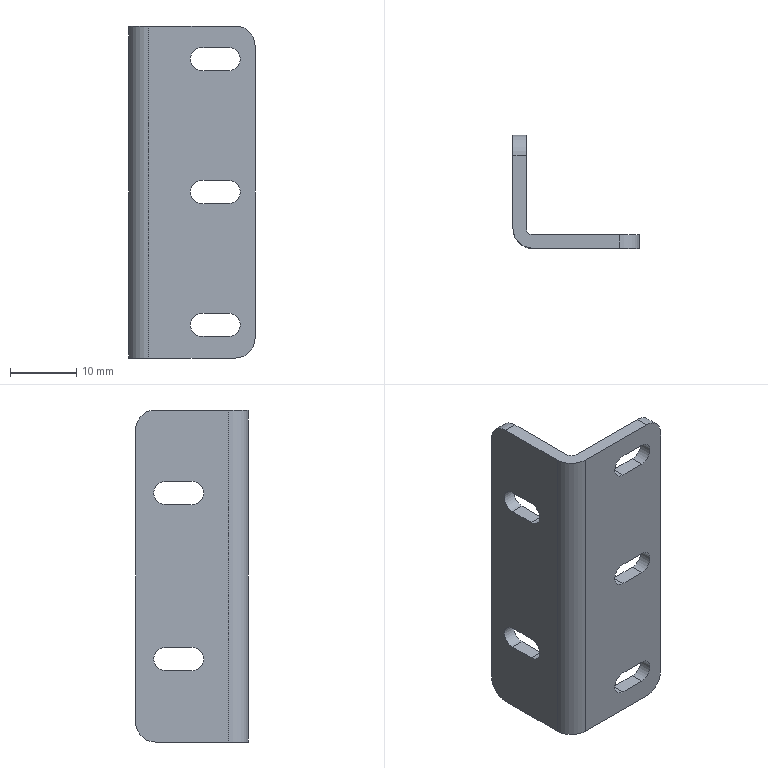Part | SolidWorks | features Fillet 3, ICE 2, ExtruThin 1 | 1 solid | 34 faces | box 19 x 17 x 50 mm | volume 3062 mm3 | plane 18 | cylinder 16 | commonest cylinder face diameters 3.5 x10 6 x5 2 x1
STEP:
#1=CARTESIAN_POINT('',(13.,-2.,18.25));
#2=VERTEX_POINT('',#1);
#3=CARTESIAN_POINT('',(9.,-2.,18.25));
#4=VERTEX_POINT('',#3);
#5=CARTESIAN_POINT('',(0.,-2.,18.25));
#6=DIRECTION('',(-1.,0.,0.));
#7=VECTOR('',#6,1000.);
#8=LINE('',#5,#7);
#9=EDGE_CURVE('',#2,#4,#8,.T.);
#10=ORIENTED_EDGE('',*,*,#9,.T.);
#11=CARTESIAN_POINT('',(9.,-2.,21.75));
#12=VERTEX_POINT('',#11);
#13=CARTESIAN_POINT('',(9.,-2.,20.));
#14=DIRECTION('',(0.,1.,0.));
#15=DIRECTION('',(0.,0.,1.));
#16=AXIS2_PLACEMENT_3D('',#13,#14,#15);
#17=CIRCLE('',#16,1.75);
#18=EDGE_CURVE('',#4,#12,#17,.T.);
#19=ORIENTED_EDGE('',*,*,#18,.T.);
#20=CARTESIAN_POINT('',(13.,-2.,21.75));
#21=VERTEX_POINT('',#20);
#22=CARTESIAN_POINT('',(0.,-2.,21.75));
#23=DIRECTION('',(1.,0.,0.));
#24=VECTOR('',#23,1000.);
#25=LINE('',#22,#24);
#26=EDGE_CURVE('',#12,#21,#25,.T.);
#27=ORIENTED_EDGE('',*,*,#26,.T.);
#28=CARTESIAN_POINT('',(13.,-2.,20.));
#29=DIRECTION('',(0.,1.,0.));
#30=DIRECTION('',(0.,0.,1.));
#31=AXIS2_PLACEMENT_3D('',#28,#29,#30);
#32=CIRCLE('',#31,1.75);
#33=EDGE_CURVE('',#21,#2,#32,.T.);
#34=ORIENTED_EDGE('',*,*,#33,.T.);
#35=EDGE_LOOP('',(#10,#19,#27,#34));
#36=FACE_BOUND('',#35,.T.);
#37=CARTESIAN_POINT('',(13.,-2.,-1.75));
#38=VERTEX_POINT('',#37);
#39=CARTESIAN_POINT('',(9.,-2.,-1.75));
#40=VERTEX_POINT('',#39);
#41=CARTESIAN_POINT('',(0.,-2.,-1.75));
#42=DIRECTION('',(-1.,0.,0.));
#43=VECTOR('',#42,1000.);
#44=LINE('',#41,#43);
#45=EDGE_CURVE('',#38,#40,#44,.T.);
#46=ORIENTED_EDGE('',*,*,#45,.T.);
#47=CARTESIAN_POINT('',(9.,-2.,1.75));
#48=VERTEX_POINT('',#47);
#49=CARTESIAN_POINT('',(9.,-2.,0.));
#50=DIRECTION('',(0.,1.,0.));
#51=DIRECTION('',(0.,0.,1.));
#52=AXIS2_PLACEMENT_3D('',#49,#50,#51);
#53=CIRCLE('',#52,1.75);
#54=EDGE_CURVE('',#40,#48,#53,.T.);
#55=ORIENTED_EDGE('',*,*,#54,.T.);
#56=CARTESIAN_POINT('',(13.,-2.,1.75));
#57=VERTEX_POINT('',#56);
#58=CARTESIAN_POINT('',(0.,-2.,1.75));
#59=DIRECTION('',(1.,0.,0.));
#60=VECTOR('',#59,1000.);
#61=LINE('',#58,#60);
#62=EDGE_CURVE('',#48,#57,#61,.T.);
#63=ORIENTED_EDGE('',*,*,#62,.T.);
#64=CARTESIAN_POINT('',(13.,-2.,0.));
#65=DIRECTION('',(0.,1.,0.));
#66=DIRECTION('',(0.,0.,1.));
#67=AXIS2_PLACEMENT_3D('',#64,#65,#66);
#68=CIRCLE('',#67,1.75);
#69=EDGE_CURVE('',#57,#38,#68,.T.);
#70=ORIENTED_EDGE('',*,*,#69,.T.);
#71=EDGE_LOOP('',(#46,#55,#63,#70));
#72=FACE_BOUND('',#71,.T.);
#73=CARTESIAN_POINT('',(13.,-2.,-21.75));
#74=VERTEX_POINT('',#73);
#75=CARTESIAN_POINT('',(9.,-2.,-21.75));
#76=VERTEX_POINT('',#75);
#77=CARTESIAN_POINT('',(0.,-2.,-21.75));
#78=DIRECTION('',(-1.,0.,0.));
#79=VECTOR('',#78,1000.);
#80=LINE('',#77,#79);
#81=EDGE_CURVE('',#74,#76,#80,.T.);
#82=ORIENTED_EDGE('',*,*,#81,.T.);
#83=CARTESIAN_POINT('',(9.,-2.,-18.25));
#84=VERTEX_POINT('',#83);
#85=CARTESIAN_POINT('',(9.,-2.,-20.));
#86=DIRECTION('',(0.,1.,0.));
#87=DIRECTION('',(0.,0.,1.));
#88=AXIS2_PLACEMENT_3D('',#85,#86,#87);
#89=CIRCLE('',#88,1.75);
#90=EDGE_CURVE('',#76,#84,#89,.T.);
#91=ORIENTED_EDGE('',*,*,#90,.T.);
#92=CARTESIAN_POINT('',(13.,-2.,-18.25));
#93=VERTEX_POINT('',#92);
#94=CARTESIAN_POINT('',(0.,-2.,-18.25));
#95=DIRECTION('',(1.,0.,0.));
#96=VECTOR('',#95,1000.);
#97=LINE('',#94,#96);
#98=EDGE_CURVE('',#84,#93,#97,.T.);
#99=ORIENTED_EDGE('',*,*,#98,.T.);
#100=CARTESIAN_POINT('',(13.,-2.,-20.));
#101=DIRECTION('',(0.,1.,0.));
#102=DIRECTION('',(0.,0.,1.));
#103=AXIS2_PLACEMENT_3D('',#100,#101,#102);
#104=CIRCLE('',#103,1.75);
#105=EDGE_CURVE('',#93,#74,#104,.T.);
#106=ORIENTED_EDGE('',*,*,#105,.T.);
#107=EDGE_LOOP('',(#82,#91,#99,#106));
#108=FACE_BOUND('',#107,.T.);
#109=CARTESIAN_POINT('',(1.,-2.,25.));
#110=VERTEX_POINT('',#109);
#111=CARTESIAN_POINT('',(14.,-2.,25.));
#112=VERTEX_POINT('',#111);
#113=CARTESIAN_POINT('',(0.,-2.,25.));
#114=DIRECTION('',(1.,0.,0.));
#115=VECTOR('',#114,1000.);
#116=LINE('',#113,#115);
#117=EDGE_CURVE('',#110,#112,#116,.T.);
#118=ORIENTED_EDGE('',*,*,#117,.F.);
#119=CARTESIAN_POINT('',(1.,-2.,-25.));
#120=VERTEX_POINT('',#119);
#121=CARTESIAN_POINT('',(1.,-2.,25.));
#122=DIRECTION('',(0.,0.,-1.));
#123=VECTOR('',#122,1000.);
#124=LINE('',#121,#123);
#125=EDGE_CURVE('',#110,#120,#124,.T.);
#126=ORIENTED_EDGE('',*,*,#125,.T.);
#127=CARTESIAN_POINT('',(14.,-2.,-25.));
#128=VERTEX_POINT('',#127);
#129=CARTESIAN_POINT('',(0.,-2.,-25.));
#130=DIRECTION('',(1.,0.,0.));
#131=VECTOR('',#130,1000.);
#132=LINE('',#129,#131);
#133=EDGE_CURVE('',#120,#128,#132,.T.);
#134=ORIENTED_EDGE('',*,*,#133,.T.);
#135=CARTESIAN_POINT('',(17.,-2.,-22.));
#136=VERTEX_POINT('',#135);
#137=CARTESIAN_POINT('',(14.,-2.,-22.));
#138=DIRECTION('',(0.,-1.,0.));
#139=DIRECTION('',(0.,0.,1.));
#140=AXIS2_PLACEMENT_3D('',#137,#138,#139);
#141=CIRCLE('',#140,3.);
#142=EDGE_CURVE('',#128,#136,#141,.T.);
#143=ORIENTED_EDGE('',*,*,#142,.T.);
#144=CARTESIAN_POINT('',(17.,-2.,22.));
#145=VERTEX_POINT('',#144);
#146=CARTESIAN_POINT('',(17.,-2.,25.));
#147=DIRECTION('',(0.,0.,-1.));
#148=VECTOR('',#147,1000.);
#149=LINE('',#146,#148);
#150=EDGE_CURVE('',#145,#136,#149,.T.);
#151=ORIENTED_EDGE('',*,*,#150,.F.);
#152=CARTESIAN_POINT('',(14.,-2.,22.));
#153=DIRECTION('',(0.,-1.,0.));
#154=DIRECTION('',(0.,0.,1.));
#155=AXIS2_PLACEMENT_3D('',#152,#153,#154);
#156=CIRCLE('',#155,3.);
#157=EDGE_CURVE('',#145,#112,#156,.T.);
#158=ORIENTED_EDGE('',*,*,#157,.T.);
#159=EDGE_LOOP('',(#118,#126,#134,#143,#151,#158));
#160=FACE_OUTER_BOUND('',#159,.T.);
#161=CARTESIAN_POINT('',(0.,-2.,25.));
#162=DIRECTION('',(0.,1.,0.));
#163=DIRECTION('',(0.,0.,1.));
#164=AXIS2_PLACEMENT_3D('',#161,#162,#163);
#165=PLANE('',#164);
#166=ADVANCED_FACE('',(#36,#72,#108,#160),#165,.F.);
#167=CARTESIAN_POINT('',(17.,0.,22.));
#168=VERTEX_POINT('',#167);
#169=CARTESIAN_POINT('',(17.,0.,-22.));
#170=VERTEX_POINT('',#169);
#171=CARTESIAN_POINT('',(17.,0.,25.));
#172=DIRECTION('',(0.,0.,-1.));
#173=VECTOR('',#172,1000.);
#174=LINE('',#171,#173);
#175=EDGE_CURVE('',#168,#170,#174,.T.);
#176=ORIENTED_EDGE('',*,*,#175,.F.);
#177=CARTESIAN_POINT('',(17.,-2.,22.));
#178=DIRECTION('',(0.,-1.,0.));
#179=VECTOR('',#178,1000.);
#180=LINE('',#177,#179);
#181=EDGE_CURVE('',#168,#145,#180,.T.);
#182=ORIENTED_EDGE('',*,*,#181,.T.);
#183=ORIENTED_EDGE('',*,*,#150,.T.);
#184=CARTESIAN_POINT('',(17.,0.,-22.));
#185=DIRECTION('',(0.,1.,0.));
#186=VECTOR('',#185,1000.);
#187=LINE('',#184,#186);
#188=EDGE_CURVE('',#136,#170,#187,.T.);
#189=ORIENTED_EDGE('',*,*,#188,.T.);
#190=EDGE_LOOP('',(#176,#182,#183,#189));
#191=FACE_OUTER_BOUND('',#190,.T.);
#192=CARTESIAN_POINT('',(17.,0.,25.));
#193=DIRECTION('',(1.,0.,0.));
#194=DIRECTION('',(0.,0.,-1.));
#195=AXIS2_PLACEMENT_3D('',#192,#193,#194);
#196=PLANE('',#195);
#197=ADVANCED_FACE('',(#191),#196,.T.);
#198=CARTESIAN_POINT('',(9.,0.,18.25));
#199=VERTEX_POINT('',#198);
#200=CARTESIAN_POINT('',(9.,0.,21.75));
#201=VERTEX_POINT('',#200);
#202=CARTESIAN_POINT('',(9.,0.,20.));
#203=DIRECTION('',(0.,1.,0.));
#204=DIRECTION('',(0.,0.,-1.));
#205=AXIS2_PLACEMENT_3D('',#202,#203,#204);
#206=CIRCLE('',#205,1.75);
#207=EDGE_CURVE('',#199,#201,#206,.T.);
#208=ORIENTED_EDGE('',*,*,#207,.F.);
#209=CARTESIAN_POINT('',(13.,0.,18.25));
#210=VERTEX_POINT('',#209);
#211=CARTESIAN_POINT('',(9.,0.,18.25));
#212=DIRECTION('',(-1.,0.,0.));
#213=VECTOR('',#212,1000.);
#214=LINE('',#211,#213);
#215=EDGE_CURVE('',#210,#199,#214,.T.);
#216=ORIENTED_EDGE('',*,*,#215,.F.);
#217=CARTESIAN_POINT('',(13.,0.,21.75));
#218=VERTEX_POINT('',#217);
#219=CARTESIAN_POINT('',(13.,0.,20.));
#220=DIRECTION('',(0.,1.,0.));
#221=DIRECTION('',(0.,0.,-1.));
#222=AXIS2_PLACEMENT_3D('',#219,#220,#221);
#223=CIRCLE('',#222,1.75);
#224=EDGE_CURVE('',#218,#210,#223,.T.);
#225=ORIENTED_EDGE('',*,*,#224,.F.);
#226=CARTESIAN_POINT('',(9.,0.,21.75));
#227=DIRECTION('',(1.,0.,0.));
#228=VECTOR('',#227,1000.);
#229=LINE('',#226,#228);
#230=EDGE_CURVE('',#201,#218,#229,.T.);
#231=ORIENTED_EDGE('',*,*,#230,.F.);
#232=EDGE_LOOP('',(#208,#216,#225,#231));
#233=FACE_BOUND('',#232,.T.);
#234=CARTESIAN_POINT('',(9.,0.,-1.75));
#235=VERTEX_POINT('',#234);
#236=CARTESIAN_POINT('',(9.,0.,1.75));
#237=VERTEX_POINT('',#236);
#238=CARTESIAN_POINT('',(9.,0.,0.));
#239=DIRECTION('',(0.,1.,0.));
#240=DIRECTION('',(0.,0.,1.));
#241=AXIS2_PLACEMENT_3D('',#238,#239,#240);
#242=CIRCLE('',#241,1.75);
#243=EDGE_CURVE('',#235,#237,#242,.T.);
#244=ORIENTED_EDGE('',*,*,#243,.F.);
#245=CARTESIAN_POINT('',(13.,0.,-1.75));
#246=VERTEX_POINT('',#245);
#247=CARTESIAN_POINT('',(9.,0.,-1.75));
#248=DIRECTION('',(-1.,0.,0.));
#249=VECTOR('',#248,1000.);
#250=LINE('',#247,#249);
#251=EDGE_CURVE('',#246,#235,#250,.T.);
#252=ORIENTED_EDGE('',*,*,#251,.F.);
#253=CARTESIAN_POINT('',(13.,0.,1.75));
#254=VERTEX_POINT('',#253);
#255=CARTESIAN_POINT('',(13.,0.,0.));
#256=DIRECTION('',(0.,1.,0.));
#257=DIRECTION('',(0.,0.,1.));
#258=AXIS2_PLACEMENT_3D('',#255,#256,#257);
#259=CIRCLE('',#258,1.75);
#260=EDGE_CURVE('',#254,#246,#259,.T.);
#261=ORIENTED_EDGE('',*,*,#260,.F.);
#262=CARTESIAN_POINT('',(9.,0.,1.75));
#263=DIRECTION('',(1.,0.,0.));
#264=VECTOR('',#263,1000.);
#265=LINE('',#262,#264);
#266=EDGE_CURVE('',#237,#254,#265,.T.);
#267=ORIENTED_EDGE('',*,*,#266,.F.);
#268=EDGE_LOOP('',(#244,#252,#261,#267));
#269=FACE_BOUND('',#268,.T.);
#270=CARTESIAN_POINT('',(9.,0.,-21.75));
#271=VERTEX_POINT('',#270);
#272=CARTESIAN_POINT('',(9.,0.,-18.25));
#273=VERTEX_POINT('',#272);
#274=CARTESIAN_POINT('',(9.,0.,-20.));
#275=DIRECTION('',(0.,1.,0.));
#276=DIRECTION('',(0.,0.,1.));
#277=AXIS2_PLACEMENT_3D('',#274,#275,#276);
#278=CIRCLE('',#277,1.75);
#279=EDGE_CURVE('',#271,#273,#278,.T.);
#280=ORIENTED_EDGE('',*,*,#279,.F.);
#281=CARTESIAN_POINT('',(13.,0.,-21.75));
#282=VERTEX_POINT('',#281);
#283=CARTESIAN_POINT('',(9.,0.,-21.75));
#284=DIRECTION('',(-1.,0.,0.));
#285=VECTOR('',#284,1000.);
#286=LINE('',#283,#285);
#287=EDGE_CURVE('',#282,#271,#286,.T.);
#288=ORIENTED_EDGE('',*,*,#287,.F.);
#289=CARTESIAN_POINT('',(13.,0.,-18.25));
#290=VERTEX_POINT('',#289);
#291=CARTESIAN_POINT('',(13.,0.,-20.));
#292=DIRECTION('',(0.,1.,0.));
#293=DIRECTION('',(0.,0.,1.));
#294=AXIS2_PLACEMENT_3D('',#291,#292,#293);
#295=CIRCLE('',#294,1.75);
#296=EDGE_CURVE('',#290,#282,#295,.T.);
#297=ORIENTED_EDGE('',*,*,#296,.F.);
#298=CARTESIAN_POINT('',(9.,0.,-18.25));
#299=DIRECTION('',(1.,0.,0.));
#300=VECTOR('',#299,1000.);
#301=LINE('',#298,#300);
#302=EDGE_CURVE('',#273,#290,#301,.T.);
#303=ORIENTED_EDGE('',*,*,#302,.F.);
#304=EDGE_LOOP('',(#280,#288,#297,#303));
#305=FACE_BOUND('',#304,.T.);
#306=CARTESIAN_POINT('',(1.,0.,-25.));
#307=VERTEX_POINT('',#306);
#308=CARTESIAN_POINT('',(14.,0.,-25.));
#309=VERTEX_POINT('',#308);
#310=CARTESIAN_POINT('',(0.,0.,-25.));
#311=DIRECTION('',(1.,0.,0.));
#312=VECTOR('',#311,1000.);
#313=LINE('',#310,#312);
#314=EDGE_CURVE('',#307,#309,#313,.T.);
#315=ORIENTED_EDGE('',*,*,#314,.F.);
#316=CARTESIAN_POINT('',(1.,0.,25.));
#317=VERTEX_POINT('',#316);
#318=CARTESIAN_POINT('',(1.,0.,25.));
#319=DIRECTION('',(0.,0.,1.));
#320=VECTOR('',#319,1000.);
#321=LINE('',#318,#320);
#322=EDGE_CURVE('',#307,#317,#321,.T.);
#323=ORIENTED_EDGE('',*,*,#322,.T.);
#324=CARTESIAN_POINT('',(14.,0.,25.));
#325=VERTEX_POINT('',#324);
#326=CARTESIAN_POINT('',(0.,0.,25.));
#327=DIRECTION('',(1.,0.,0.));
#328=VECTOR('',#327,1000.);
#329=LINE('',#326,#328);
#330=EDGE_CURVE('',#317,#325,#329,.T.);
#331=ORIENTED_EDGE('',*,*,#330,.T.);
#332=CARTESIAN_POINT('',(14.,0.,22.));
#333=DIRECTION('',(0.,1.,0.));
#334=DIRECTION('',(0.,0.,1.));
#335=AXIS2_PLACEMENT_3D('',#332,#333,#334);
#336=CIRCLE('',#335,3.);
#337=EDGE_CURVE('',#325,#168,#336,.T.);
#338=ORIENTED_EDGE('',*,*,#337,.T.);
#339=ORIENTED_EDGE('',*,*,#175,.T.);
#340=CARTESIAN_POINT('',(14.,0.,-22.));
#341=DIRECTION('',(0.,1.,0.));
#342=DIRECTION('',(0.,0.,1.));
#343=AXIS2_PLACEMENT_3D('',#340,#341,#342);
#344=CIRCLE('',#343,3.);
#345=EDGE_CURVE('',#170,#309,#344,.T.);
#346=ORIENTED_EDGE('',*,*,#345,.T.);
#347=EDGE_LOOP('',(#315,#323,#331,#338,#339,#346));
#348=FACE_OUTER_BOUND('',#347,.T.);
#349=CARTESIAN_POINT('',(0.,0.,25.));
#350=DIRECTION('',(0.,1.,0.));
#351=DIRECTION('',(0.,0.,1.));
#352=AXIS2_PLACEMENT_3D('',#349,#350,#351);
#353=PLANE('',#352);
#354=ADVANCED_FACE('',(#233,#269,#305,#348),#353,.T.);
#355=CARTESIAN_POINT('',(0.,10.5,-14.25));
#356=VERTEX_POINT('',#355);
#357=CARTESIAN_POINT('',(0.,10.5,-10.75));
#358=VERTEX_POINT('',#357);
#359=CARTESIAN_POINT('',(0.,10.5,-12.5));
#360=DIRECTION('',(1.,0.,0.));
#361=DIRECTION('',(0.,0.,1.));
#362=AXIS2_PLACEMENT_3D('',#359,#360,#361);
#363=CIRCLE('',#362,1.75);
#364=EDGE_CURVE('',#356,#358,#363,.T.);
#365=ORIENTED_EDGE('',*,*,#364,.F.);
#366=CARTESIAN_POINT('',(0.,6.5,-14.25));
#367=VERTEX_POINT('',#366);
#368=CARTESIAN_POINT('',(0.,10.5,-14.25));
#369=DIRECTION('',(0.,1.,0.));
#370=VECTOR('',#369,1000.);
#371=LINE('',#368,#370);
#372=EDGE_CURVE('',#367,#356,#371,.T.);
#373=ORIENTED_EDGE('',*,*,#372,.F.);
#374=CARTESIAN_POINT('',(0.,6.5,-10.75));
#375=VERTEX_POINT('',#374);
#376=CARTESIAN_POINT('',(0.,6.5,-12.5));
#377=DIRECTION('',(1.,0.,0.));
#378=DIRECTION('',(0.,0.,1.));
#379=AXIS2_PLACEMENT_3D('',#376,#377,#378);
#380=CIRCLE('',#379,1.75);
#381=EDGE_CURVE('',#375,#367,#380,.T.);
#382=ORIENTED_EDGE('',*,*,#381,.F.);
#383=CARTESIAN_POINT('',(0.,10.5,-10.75));
#384=DIRECTION('',(0.,-1.,0.));
#385=VECTOR('',#384,1000.);
#386=LINE('',#383,#385);
#387=EDGE_CURVE('',#358,#375,#386,.T.);
#388=ORIENTED_EDGE('',*,*,#387,.F.);
#389=EDGE_LOOP('',(#365,#373,#382,#388));
#390=FACE_BOUND('',#389,.T.);
#391=CARTESIAN_POINT('',(0.,10.5,10.75));
#392=VERTEX_POINT('',#391);
#393=CARTESIAN_POINT('',(0.,10.5,14.25));
#394=VERTEX_POINT('',#393);
#395=CARTESIAN_POINT('',(0.,10.5,12.5));
#396=DIRECTION('',(1.,0.,0.));
#397=DIRECTION('',(0.,0.,-1.));
#398=AXIS2_PLACEMENT_3D('',#395,#396,#397);
#399=CIRCLE('',#398,1.75);
#400=EDGE_CURVE('',#392,#394,#399,.T.);
#401=ORIENTED_EDGE('',*,*,#400,.F.);
#402=CARTESIAN_POINT('',(0.,6.5,10.75));
#403=VERTEX_POINT('',#402);
#404=CARTESIAN_POINT('',(0.,10.5,10.75));
#405=DIRECTION('',(0.,1.,0.));
#406=VECTOR('',#405,1000.);
#407=LINE('',#404,#406);
#408=EDGE_CURVE('',#403,#392,#407,.T.);
#409=ORIENTED_EDGE('',*,*,#408,.F.);
#410=CARTESIAN_POINT('',(0.,6.5,14.25));
#411=VERTEX_POINT('',#410);
#412=CARTESIAN_POINT('',(0.,6.5,12.5));
#413=DIRECTION('',(1.,0.,0.));
#414=DIRECTION('',(0.,0.,-1.));
#415=AXIS2_PLACEMENT_3D('',#412,#413,#414);
#416=CIRCLE('',#415,1.75);
#417=EDGE_CURVE('',#411,#403,#416,.T.);
#418=ORIENTED_EDGE('',*,*,#417,.F.);
#419=CARTESIAN_POINT('',(0.,10.5,14.25));
#420=DIRECTION('',(0.,-1.,0.));
#421=VECTOR('',#420,1000.);
#422=LINE('',#419,#421);
#423=EDGE_CURVE('',#394,#411,#422,.T.);
#424=ORIENTED_EDGE('',*,*,#423,.F.);
#425=EDGE_LOOP('',(#401,#409,#418,#424));
#426=FACE_BOUND('',#425,.T.);
#427=CARTESIAN_POINT('',(0.,12.,25.));
#428=VERTEX_POINT('',#427);
#429=CARTESIAN_POINT('',(0.,1.,25.));
#430=VERTEX_POINT('',#429);
#431=CARTESIAN_POINT('',(0.,0.,25.));
#432=DIRECTION('',(0.,-1.,0.));
#433=VECTOR('',#432,1000.);
#434=LINE('',#431,#433);
#435=EDGE_CURVE('',#428,#430,#434,.T.);
#436=ORIENTED_EDGE('',*,*,#435,.T.);
#437=CARTESIAN_POINT('',(0.,1.,-25.));
#438=VERTEX_POINT('',#437);
#439=CARTESIAN_POINT('',(0.,1.,-25.));
#440=DIRECTION('',(0.,0.,-1.));
#441=VECTOR('',#440,1000.);
#442=LINE('',#439,#441);
#443=EDGE_CURVE('',#430,#438,#442,.T.);
#444=ORIENTED_EDGE('',*,*,#443,.T.);
#445=CARTESIAN_POINT('',(0.,12.,-25.));
#446=VERTEX_POINT('',#445);
#447=CARTESIAN_POINT('',(0.,0.,-25.));
#448=DIRECTION('',(0.,-1.,0.));
#449=VECTOR('',#448,1000.);
#450=LINE('',#447,#449);
#451=EDGE_CURVE('',#446,#438,#450,.T.);
#452=ORIENTED_EDGE('',*,*,#451,.F.);
#453=CARTESIAN_POINT('',(0.,15.,-22.));
#454=VERTEX_POINT('',#453);
#455=CARTESIAN_POINT('',(0.,12.,-22.));
#456=DIRECTION('',(1.,0.,0.));
#457=DIRECTION('',(0.,0.,-1.));
#458=AXIS2_PLACEMENT_3D('',#455,#456,#457);
#459=CIRCLE('',#458,3.);
#460=EDGE_CURVE('',#446,#454,#459,.T.);
#461=ORIENTED_EDGE('',*,*,#460,.T.);
#462=CARTESIAN_POINT('',(0.,15.,22.));
#463=VERTEX_POINT('',#462);
#464=CARTESIAN_POINT('',(0.,15.,25.));
#465=DIRECTION('',(0.,0.,-1.));
#466=VECTOR('',#465,1000.);
#467=LINE('',#464,#466);
#468=EDGE_CURVE('',#463,#454,#467,.T.);
#469=ORIENTED_EDGE('',*,*,#468,.F.);
#470=CARTESIAN_POINT('',(0.,12.,22.));
#471=DIRECTION('',(1.,0.,0.));
#472=DIRECTION('',(0.,0.,-1.));
#473=AXIS2_PLACEMENT_3D('',#470,#471,#472);
#474=CIRCLE('',#473,3.);
#475=EDGE_CURVE('',#463,#428,#474,.T.);
#476=ORIENTED_EDGE('',*,*,#475,.T.);
#477=EDGE_LOOP('',(#436,#444,#452,#461,#469,#476));
#478=FACE_OUTER_BOUND('',#477,.T.);
#479=CARTESIAN_POINT('',(0.,0.,25.));
#480=DIRECTION('',(1.,0.,0.));
#481=DIRECTION('',(0.,0.,-1.));
#482=AXIS2_PLACEMENT_3D('',#479,#480,#481);
#483=PLANE('',#482);
#484=ADVANCED_FACE('',(#390,#426,#478),#483,.T.);
#485=CARTESIAN_POINT('',(-2.,15.,22.));
#486=VERTEX_POINT('',#485);
#487=CARTESIAN_POINT('',(-2.,15.,-22.));
#488=VERTEX_POINT('',#487);
#489=CARTESIAN_POINT('',(-2.,15.,25.));
#490=DIRECTION('',(0.,0.,-1.));
#491=VECTOR('',#490,1000.);
#492=LINE('',#489,#491);
#493=EDGE_CURVE('',#486,#488,#492,.T.);
#494=ORIENTED_EDGE('',*,*,#493,.F.);
#495=CARTESIAN_POINT('',(0.,15.,22.));
#496=DIRECTION('',(1.,0.,0.));
#497=VECTOR('',#496,1000.);
#498=LINE('',#495,#497);
#499=EDGE_CURVE('',#486,#463,#498,.T.);
#500=ORIENTED_EDGE('',*,*,#499,.T.);
#501=ORIENTED_EDGE('',*,*,#468,.T.);
#502=CARTESIAN_POINT('',(-2.,15.,-22.));
#503=DIRECTION('',(-1.,0.,0.));
#504=VECTOR('',#503,1000.);
#505=LINE('',#502,#504);
#506=EDGE_CURVE('',#454,#488,#505,.T.);
#507=ORIENTED_EDGE('',*,*,#506,.T.);
#508=EDGE_LOOP('',(#494,#500,#501,#507));
#509=FACE_OUTER_BOUND('',#508,.T.);
#510=CARTESIAN_POINT('',(-2.,15.,25.));
#511=DIRECTION('',(0.,1.,0.));
#512=DIRECTION('',(0.,0.,1.));
#513=AXIS2_PLACEMENT_3D('',#510,#511,#512);
#514=PLANE('',#513);
#515=ADVANCED_FACE('',(#509),#514,.T.);
#516=CARTESIAN_POINT('',(-2.,6.5,-14.25));
#517=VERTEX_POINT('',#516);
#518=CARTESIAN_POINT('',(-2.,10.5,-14.25));
#519=VERTEX_POINT('',#518);
#520=CARTESIAN_POINT('',(-2.,0.,-14.25));
#521=DIRECTION('',(0.,1.,0.));
#522=VECTOR('',#521,1000.);
#523=LINE('',#520,#522);
#524=EDGE_CURVE('',#517,#519,#523,.T.);
#525=ORIENTED_EDGE('',*,*,#524,.T.);
#526=CARTESIAN_POINT('',(-2.,10.5,-10.75));
#527=VERTEX_POINT('',#526);
#528=CARTESIAN_POINT('',(-2.,10.5,-12.5));
#529=DIRECTION('',(1.,0.,0.));
#530=DIRECTION('',(0.,0.,-1.));
#531=AXIS2_PLACEMENT_3D('',#528,#529,#530);
#532=CIRCLE('',#531,1.75);
#533=EDGE_CURVE('',#519,#527,#532,.T.);
#534=ORIENTED_EDGE('',*,*,#533,.T.);
#535=CARTESIAN_POINT('',(-2.,6.5,-10.75));
#536=VERTEX_POINT('',#535);
#537=CARTESIAN_POINT('',(-2.,0.,-10.75));
#538=DIRECTION('',(0.,-1.,0.));
#539=VECTOR('',#538,1000.);
#540=LINE('',#537,#539);
#541=EDGE_CURVE('',#527,#536,#540,.T.);
#542=ORIENTED_EDGE('',*,*,#541,.T.);
#543=CARTESIAN_POINT('',(-2.,6.5,-12.5));
#544=DIRECTION('',(1.,0.,0.));
#545=DIRECTION('',(0.,0.,-1.));
#546=AXIS2_PLACEMENT_3D('',#543,#544,#545);
#547=CIRCLE('',#546,1.75);
#548=EDGE_CURVE('',#536,#517,#547,.T.);
#549=ORIENTED_EDGE('',*,*,#548,.T.);
#550=EDGE_LOOP('',(#525,#534,#542,#549));
#551=FACE_BOUND('',#550,.T.);
#552=CARTESIAN_POINT('',(-2.,6.5,10.75));
#553=VERTEX_POINT('',#552);
#554=CARTESIAN_POINT('',(-2.,10.5,10.75));
#555=VERTEX_POINT('',#554);
#556=CARTESIAN_POINT('',(-2.,0.,10.75));
#557=DIRECTION('',(0.,1.,0.));
#558=VECTOR('',#557,1000.);
#559=LINE('',#556,#558);
#560=EDGE_CURVE('',#553,#555,#559,.T.);
#561=ORIENTED_EDGE('',*,*,#560,.T.);
#562=CARTESIAN_POINT('',(-2.,10.5,14.25));
#563=VERTEX_POINT('',#562);
#564=CARTESIAN_POINT('',(-2.,10.5,12.5));
#565=DIRECTION('',(1.,0.,0.));
#566=DIRECTION('',(0.,0.,-1.));
#567=AXIS2_PLACEMENT_3D('',#564,#565,#566);
#568=CIRCLE('',#567,1.75);
#569=EDGE_CURVE('',#555,#563,#568,.T.);
#570=ORIENTED_EDGE('',*,*,#569,.T.);
#571=CARTESIAN_POINT('',(-2.,6.5,14.25));
#572=VERTEX_POINT('',#571);
#573=CARTESIAN_POINT('',(-2.,0.,14.25));
#574=DIRECTION('',(0.,-1.,0.));
#575=VECTOR('',#574,1000.);
#576=LINE('',#573,#575);
#577=EDGE_CURVE('',#563,#572,#576,.T.);
#578=ORIENTED_EDGE('',*,*,#577,.T.);
#579=CARTESIAN_POINT('',(-2.,6.5,12.5));
#580=DIRECTION('',(1.,0.,0.));
#581=DIRECTION('',(0.,0.,-1.));
#582=AXIS2_PLACEMENT_3D('',#579,#580,#581);
#583=CIRCLE('',#582,1.75);
#584=EDGE_CURVE('',#572,#553,#583,.T.);
#585=ORIENTED_EDGE('',*,*,#584,.T.);
#586=EDGE_LOOP('',(#561,#570,#578,#585));
#587=FACE_BOUND('',#586,.T.);
#588=CARTESIAN_POINT('',(-2.,12.,-25.));
#589=VERTEX_POINT('',#588);
#590=CARTESIAN_POINT('',(-2.,1.,-25.));
#591=VERTEX_POINT('',#590);
#592=CARTESIAN_POINT('',(-2.,0.,-25.));
#593=DIRECTION('',(0.,-1.,0.));
#594=VECTOR('',#593,1000.);
#595=LINE('',#592,#594);
#596=EDGE_CURVE('',#589,#591,#595,.T.);
#597=ORIENTED_EDGE('',*,*,#596,.T.);
#598=CARTESIAN_POINT('',(-2.,1.,25.));
#599=VERTEX_POINT('',#598);
#600=CARTESIAN_POINT('',(-2.,1.,25.));
#601=DIRECTION('',(0.,0.,1.));
#602=VECTOR('',#601,1000.);
#603=LINE('',#600,#602);
#604=EDGE_CURVE('',#591,#599,#603,.T.);
#605=ORIENTED_EDGE('',*,*,#604,.T.);
#606=CARTESIAN_POINT('',(-2.,12.,25.));
#607=VERTEX_POINT('',#606);
#608=CARTESIAN_POINT('',(-2.,0.,25.));
#609=DIRECTION('',(0.,-1.,0.));
#610=VECTOR('',#609,1000.);
#611=LINE('',#608,#610);
#612=EDGE_CURVE('',#607,#599,#611,.T.);
#613=ORIENTED_EDGE('',*,*,#612,.F.);
#614=CARTESIAN_POINT('',(-2.,12.,22.));
#615=DIRECTION('',(-1.,0.,0.));
#616=DIRECTION('',(0.,0.,-1.));
#617=AXIS2_PLACEMENT_3D('',#614,#615,#616);
#618=CIRCLE('',#617,3.);
#619=EDGE_CURVE('',#607,#486,#618,.T.);
#620=ORIENTED_EDGE('',*,*,#619,.T.);
#621=ORIENTED_EDGE('',*,*,#493,.T.);
#622=CARTESIAN_POINT('',(-2.,12.,-22.));
#623=DIRECTION('',(-1.,0.,0.));
#624=DIRECTION('',(0.,0.,-1.));
#625=AXIS2_PLACEMENT_3D('',#622,#623,#624);
#626=CIRCLE('',#625,3.);
#627=EDGE_CURVE('',#488,#589,#626,.T.);
#628=ORIENTED_EDGE('',*,*,#627,.T.);
#629=EDGE_LOOP('',(#597,#605,#613,#620,#621,#628));
#630=FACE_OUTER_BOUND('',#629,.T.);
#631=CARTESIAN_POINT('',(-2.,0.,25.));
#632=DIRECTION('',(1.,0.,0.));
#633=DIRECTION('',(0.,0.,-1.));
#634=AXIS2_PLACEMENT_3D('',#631,#632,#633);
#635=PLANE('',#634);
#636=ADVANCED_FACE('',(#551,#587,#630),#635,.F.);
#637=ORIENTED_EDGE('',*,*,#612,.T.);
#638=CARTESIAN_POINT('',(1.,1.,25.));
#639=DIRECTION('',(0.,0.,1.));
#640=DIRECTION('',(-1.,0.,0.));
#641=AXIS2_PLACEMENT_3D('',#638,#639,#640);
#642=CIRCLE('',#641,3.);
#643=EDGE_CURVE('',#599,#110,#642,.T.);
#644=ORIENTED_EDGE('',*,*,#643,.T.);
#645=ORIENTED_EDGE('',*,*,#117,.T.);
#646=CARTESIAN_POINT('',(14.,0.,25.));
#647=DIRECTION('',(0.,1.,0.));
#648=VECTOR('',#647,1000.);
#649=LINE('',#646,#648);
#650=EDGE_CURVE('',#112,#325,#649,.T.);
#651=ORIENTED_EDGE('',*,*,#650,.T.);
#652=ORIENTED_EDGE('',*,*,#330,.F.);
#653=CARTESIAN_POINT('',(1.,1.,25.));
#654=DIRECTION('',(0.,0.,-1.));
#655=DIRECTION('',(-1.,0.,0.));
#656=AXIS2_PLACEMENT_3D('',#653,#654,#655);
#657=CIRCLE('',#656,1.);
#658=EDGE_CURVE('',#317,#430,#657,.T.);
#659=ORIENTED_EDGE('',*,*,#658,.T.);
#660=ORIENTED_EDGE('',*,*,#435,.F.);
#661=CARTESIAN_POINT('',(-2.,12.,25.));
#662=DIRECTION('',(-1.,0.,0.));
#663=VECTOR('',#662,1000.);
#664=LINE('',#661,#663);
#665=EDGE_CURVE('',#428,#607,#664,.T.);
#666=ORIENTED_EDGE('',*,*,#665,.T.);
#667=EDGE_LOOP('',(#637,#644,#645,#651,#652,#659,#660,#666));
#668=FACE_OUTER_BOUND('',#667,.T.);
#669=CARTESIAN_POINT('',(0.,0.,25.));
#670=DIRECTION('',(0.,0.,-1.));
#671=DIRECTION('',(-1.,0.,0.));
#672=AXIS2_PLACEMENT_3D('',#669,#670,#671);
#673=PLANE('',#672);
#674=ADVANCED_FACE('',(#668),#673,.F.);
#675=ORIENTED_EDGE('',*,*,#133,.F.);
#676=CARTESIAN_POINT('',(1.,1.,-25.));
#677=DIRECTION('',(0.,0.,-1.));
#678=DIRECTION('',(-1.,0.,0.));
#679=AXIS2_PLACEMENT_3D('',#676,#677,#678);
#680=CIRCLE('',#679,3.);
#681=EDGE_CURVE('',#120,#591,#680,.T.);
#682=ORIENTED_EDGE('',*,*,#681,.T.);
#683=ORIENTED_EDGE('',*,*,#596,.F.);
#684=CARTESIAN_POINT('',(0.,12.,-25.));
#685=DIRECTION('',(1.,0.,0.));
#686=VECTOR('',#685,1000.);
#687=LINE('',#684,#686);
#688=EDGE_CURVE('',#589,#446,#687,.T.);
#689=ORIENTED_EDGE('',*,*,#688,.T.);
#690=ORIENTED_EDGE('',*,*,#451,.T.);
#691=CARTESIAN_POINT('',(1.,1.,-25.));
#692=DIRECTION('',(0.,0.,1.));
#693=DIRECTION('',(-1.,0.,0.));
#694=AXIS2_PLACEMENT_3D('',#691,#692,#693);
#695=CIRCLE('',#694,1.);
#696=EDGE_CURVE('',#438,#307,#695,.T.);
#697=ORIENTED_EDGE('',*,*,#696,.T.);
#698=ORIENTED_EDGE('',*,*,#314,.T.);
#699=CARTESIAN_POINT('',(14.,0.,-25.));
#700=DIRECTION('',(0.,-1.,0.));
#701=VECTOR('',#700,1000.);
#702=LINE('',#699,#701);
#703=EDGE_CURVE('',#309,#128,#702,.T.);
#704=ORIENTED_EDGE('',*,*,#703,.T.);
#705=EDGE_LOOP('',(#675,#682,#683,#689,#690,#697,#698,#704));
#706=FACE_OUTER_BOUND('',#705,.T.);
#707=CARTESIAN_POINT('',(0.,0.,-25.));
#708=DIRECTION('',(0.,0.,-1.));
#709=DIRECTION('',(-1.,0.,0.));
#710=AXIS2_PLACEMENT_3D('',#707,#708,#709);
#711=PLANE('',#710);
#712=ADVANCED_FACE('',(#706),#711,.T.);
#713=CARTESIAN_POINT('',(9.,-10.,-21.75));
#714=DIRECTION('',(0.,1.,0.));
#715=VECTOR('',#714,1000.);
#716=LINE('',#713,#715);
#717=EDGE_CURVE('',#76,#271,#716,.T.);
#718=ORIENTED_EDGE('',*,*,#717,.T.);
#719=ORIENTED_EDGE('',*,*,#279,.T.);
#720=CARTESIAN_POINT('',(9.,-10.,-18.25));
#721=DIRECTION('',(0.,1.,0.));
#722=VECTOR('',#721,1000.);
#723=LINE('',#720,#722);
#724=EDGE_CURVE('',#84,#273,#723,.T.);
#725=ORIENTED_EDGE('',*,*,#724,.F.);
#726=ORIENTED_EDGE('',*,*,#90,.F.);
#727=EDGE_LOOP('',(#718,#719,#725,#726));
#728=FACE_OUTER_BOUND('',#727,.T.);
#729=CARTESIAN_POINT('',(9.,-10.,-20.));
#730=DIRECTION('',(0.,1.,0.));
#731=DIRECTION('',(0.,0.,1.));
#732=AXIS2_PLACEMENT_3D('',#729,#730,#731);
#733=CYLINDRICAL_SURFACE('',#732,1.75);
#734=ADVANCED_FACE('',(#728),#733,.F.);
#735=CARTESIAN_POINT('',(13.,-10.,-21.75));
#736=DIRECTION('',(0.,1.,0.));
#737=VECTOR('',#736,1000.);
#738=LINE('',#735,#737);
#739=EDGE_CURVE('',#74,#282,#738,.T.);
#740=ORIENTED_EDGE('',*,*,#739,.T.);
#741=ORIENTED_EDGE('',*,*,#287,.T.);
#742=ORIENTED_EDGE('',*,*,#717,.F.);
#743=ORIENTED_EDGE('',*,*,#81,.F.);
#744=EDGE_LOOP('',(#740,#741,#742,#743));
#745=FACE_OUTER_BOUND('',#744,.T.);
#746=CARTESIAN_POINT('',(9.,-10.,-21.75));
#747=DIRECTION('',(0.,0.,-1.));
#748=DIRECTION('',(-1.,0.,0.));
#749=AXIS2_PLACEMENT_3D('',#746,#747,#748);
#750=PLANE('',#749);
#751=ADVANCED_FACE('',(#745),#750,.F.);
#752=CARTESIAN_POINT('',(13.,-10.,-18.25));
#753=DIRECTION('',(0.,1.,0.));
#754=VECTOR('',#753,1000.);
#755=LINE('',#752,#754);
#756=EDGE_CURVE('',#93,#290,#755,.T.);
#757=ORIENTED_EDGE('',*,*,#756,.T.);
#758=ORIENTED_EDGE('',*,*,#296,.T.);
#759=ORIENTED_EDGE('',*,*,#739,.F.);
#760=ORIENTED_EDGE('',*,*,#105,.F.);
#761=EDGE_LOOP('',(#757,#758,#759,#760));
#762=FACE_OUTER_BOUND('',#761,.T.);
#763=CARTESIAN_POINT('',(13.,-10.,-20.));
#764=DIRECTION('',(0.,1.,0.));
#765=DIRECTION('',(0.,0.,1.));
#766=AXIS2_PLACEMENT_3D('',#763,#764,#765);
#767=CYLINDRICAL_SURFACE('',#766,1.75);
#768=ADVANCED_FACE('',(#762),#767,.F.);
#769=ORIENTED_EDGE('',*,*,#724,.T.);
#770=ORIENTED_EDGE('',*,*,#302,.T.);
#771=ORIENTED_EDGE('',*,*,#756,.F.);
#772=ORIENTED_EDGE('',*,*,#98,.F.);
#773=EDGE_LOOP('',(#769,#770,#771,#772));
#774=FACE_OUTER_BOUND('',#773,.T.);
#775=CARTESIAN_POINT('',(9.,-10.,-18.25));
#776=DIRECTION('',(0.,0.,1.));
#777=DIRECTION('',(1.,0.,0.));
#778=AXIS2_PLACEMENT_3D('',#775,#776,#777);
#779=PLANE('',#778);
#780=ADVANCED_FACE('',(#774),#779,.F.);
#781=CARTESIAN_POINT('',(9.,-10.,-1.75));
#782=DIRECTION('',(0.,1.,0.));
#783=VECTOR('',#782,1000.);
#784=LINE('',#781,#783);
#785=EDGE_CURVE('',#40,#235,#784,.T.);
#786=ORIENTED_EDGE('',*,*,#785,.T.);
#787=ORIENTED_EDGE('',*,*,#243,.T.);
#788=CARTESIAN_POINT('',(9.,-10.,1.75));
#789=DIRECTION('',(0.,1.,0.));
#790=VECTOR('',#789,1000.);
#791=LINE('',#788,#790);
#792=EDGE_CURVE('',#48,#237,#791,.T.);
#793=ORIENTED_EDGE('',*,*,#792,.F.);
#794=ORIENTED_EDGE('',*,*,#54,.F.);
#795=EDGE_LOOP('',(#786,#787,#793,#794));
#796=FACE_OUTER_BOUND('',#795,.T.);
#797=CARTESIAN_POINT('',(9.,-10.,0.));
#798=DIRECTION('',(0.,1.,0.));
#799=DIRECTION('',(0.,0.,1.));
#800=AXIS2_PLACEMENT_3D('',#797,#798,#799);
#801=CYLINDRICAL_SURFACE('',#800,1.75);
#802=ADVANCED_FACE('',(#796),#801,.F.);
#803=CARTESIAN_POINT('',(13.,-10.,-1.75));
#804=DIRECTION('',(0.,1.,0.));
#805=VECTOR('',#804,1000.);
#806=LINE('',#803,#805);
#807=EDGE_CURVE('',#38,#246,#806,.T.);
#808=ORIENTED_EDGE('',*,*,#807,.T.);
#809=ORIENTED_EDGE('',*,*,#251,.T.);
#810=ORIENTED_EDGE('',*,*,#785,.F.);
#811=ORIENTED_EDGE('',*,*,#45,.F.);
#812=EDGE_LOOP('',(#808,#809,#810,#811));
#813=FACE_OUTER_BOUND('',#812,.T.);
#814=CARTESIAN_POINT('',(9.,-10.,-1.75));
#815=DIRECTION('',(0.,0.,-1.));
#816=DIRECTION('',(-1.,0.,0.));
#817=AXIS2_PLACEMENT_3D('',#814,#815,#816);
#818=PLANE('',#817);
#819=ADVANCED_FACE('',(#813),#818,.F.);
#820=CARTESIAN_POINT('',(13.,-10.,1.75));
#821=DIRECTION('',(0.,1.,0.));
#822=VECTOR('',#821,1000.);
#823=LINE('',#820,#822);
#824=EDGE_CURVE('',#57,#254,#823,.T.);
#825=ORIENTED_EDGE('',*,*,#824,.T.);
#826=ORIENTED_EDGE('',*,*,#260,.T.);
#827=ORIENTED_EDGE('',*,*,#807,.F.);
#828=ORIENTED_EDGE('',*,*,#69,.F.);
#829=EDGE_LOOP('',(#825,#826,#827,#828));
#830=FACE_OUTER_BOUND('',#829,.T.);
#831=CARTESIAN_POINT('',(13.,-10.,0.));
#832=DIRECTION('',(0.,1.,0.));
#833=DIRECTION('',(0.,0.,1.));
#834=AXIS2_PLACEMENT_3D('',#831,#832,#833);
#835=CYLINDRICAL_SURFACE('',#834,1.75);
#836=ADVANCED_FACE('',(#830),#835,.F.);
#837=ORIENTED_EDGE('',*,*,#792,.T.);
#838=ORIENTED_EDGE('',*,*,#266,.T.);
#839=ORIENTED_EDGE('',*,*,#824,.F.);
#840=ORIENTED_EDGE('',*,*,#62,.F.);
#841=EDGE_LOOP('',(#837,#838,#839,#840));
#842=FACE_OUTER_BOUND('',#841,.T.);
#843=CARTESIAN_POINT('',(9.,-10.,1.75));
#844=DIRECTION('',(0.,0.,1.));
#845=DIRECTION('',(1.,0.,0.));
#846=AXIS2_PLACEMENT_3D('',#843,#844,#845);
#847=PLANE('',#846);
#848=ADVANCED_FACE('',(#842),#847,.F.);
#849=CARTESIAN_POINT('',(9.,-10.,18.25));
#850=DIRECTION('',(0.,1.,0.));
#851=VECTOR('',#850,1000.);
#852=LINE('',#849,#851);
#853=EDGE_CURVE('',#4,#199,#852,.T.);
#854=ORIENTED_EDGE('',*,*,#853,.T.);
#855=ORIENTED_EDGE('',*,*,#207,.T.);
#856=CARTESIAN_POINT('',(9.,-10.,21.75));
#857=DIRECTION('',(0.,1.,0.));
#858=VECTOR('',#857,1000.);
#859=LINE('',#856,#858);
#860=EDGE_CURVE('',#12,#201,#859,.T.);
#861=ORIENTED_EDGE('',*,*,#860,.F.);
#862=ORIENTED_EDGE('',*,*,#18,.F.);
#863=EDGE_LOOP('',(#854,#855,#861,#862));
#864=FACE_OUTER_BOUND('',#863,.T.);
#865=CARTESIAN_POINT('',(9.,-10.,20.));
#866=DIRECTION('',(0.,1.,0.));
#867=DIRECTION('',(0.,0.,1.));
#868=AXIS2_PLACEMENT_3D('',#865,#866,#867);
#869=CYLINDRICAL_SURFACE('',#868,1.75);
#870=ADVANCED_FACE('',(#864),#869,.F.);
#871=CARTESIAN_POINT('',(13.,-10.,18.25));
#872=DIRECTION('',(0.,1.,0.));
#873=VECTOR('',#872,1000.);
#874=LINE('',#871,#873);
#875=EDGE_CURVE('',#2,#210,#874,.T.);
#876=ORIENTED_EDGE('',*,*,#875,.T.);
#877=ORIENTED_EDGE('',*,*,#215,.T.);
#878=ORIENTED_EDGE('',*,*,#853,.F.);
#879=ORIENTED_EDGE('',*,*,#9,.F.);
#880=EDGE_LOOP('',(#876,#877,#878,#879));
#881=FACE_OUTER_BOUND('',#880,.T.);
#882=CARTESIAN_POINT('',(9.,-10.,18.25));
#883=DIRECTION('',(0.,0.,-1.));
#884=DIRECTION('',(-1.,0.,0.));
#885=AXIS2_PLACEMENT_3D('',#882,#883,#884);
#886=PLANE('',#885);
#887=ADVANCED_FACE('',(#881),#886,.F.);
#888=CARTESIAN_POINT('',(13.,-10.,21.75));
#889=DIRECTION('',(0.,1.,0.));
#890=VECTOR('',#889,1000.);
#891=LINE('',#888,#890);
#892=EDGE_CURVE('',#21,#218,#891,.T.);
#893=ORIENTED_EDGE('',*,*,#892,.T.);
#894=ORIENTED_EDGE('',*,*,#224,.T.);
#895=ORIENTED_EDGE('',*,*,#875,.F.);
#896=ORIENTED_EDGE('',*,*,#33,.F.);
#897=EDGE_LOOP('',(#893,#894,#895,#896));
#898=FACE_OUTER_BOUND('',#897,.T.);
#899=CARTESIAN_POINT('',(13.,-10.,20.));
#900=DIRECTION('',(0.,1.,0.));
#901=DIRECTION('',(0.,0.,1.));
#902=AXIS2_PLACEMENT_3D('',#899,#900,#901);
#903=CYLINDRICAL_SURFACE('',#902,1.75);
#904=ADVANCED_FACE('',(#898),#903,.F.);
#905=ORIENTED_EDGE('',*,*,#860,.T.);
#906=ORIENTED_EDGE('',*,*,#230,.T.);
#907=ORIENTED_EDGE('',*,*,#892,.F.);
#908=ORIENTED_EDGE('',*,*,#26,.F.);
#909=EDGE_LOOP('',(#905,#906,#907,#908));
#910=FACE_OUTER_BOUND('',#909,.T.);
#911=CARTESIAN_POINT('',(9.,-10.,21.75));
#912=DIRECTION('',(0.,0.,1.));
#913=DIRECTION('',(1.,0.,0.));
#914=AXIS2_PLACEMENT_3D('',#911,#912,#913);
#915=PLANE('',#914);
#916=ADVANCED_FACE('',(#910),#915,.F.);
#917=CARTESIAN_POINT('',(-10.,10.5,10.75));
#918=DIRECTION('',(1.,0.,0.));
#919=VECTOR('',#918,1000.);
#920=LINE('',#917,#919);
#921=EDGE_CURVE('',#555,#392,#920,.T.);
#922=ORIENTED_EDGE('',*,*,#921,.T.);
#923=ORIENTED_EDGE('',*,*,#400,.T.);
#924=CARTESIAN_POINT('',(-10.,10.5,14.25));
#925=DIRECTION('',(1.,0.,0.));
#926=VECTOR('',#925,1000.);
#927=LINE('',#924,#926);
#928=EDGE_CURVE('',#563,#394,#927,.T.);
#929=ORIENTED_EDGE('',*,*,#928,.F.);
#930=ORIENTED_EDGE('',*,*,#569,.F.);
#931=EDGE_LOOP('',(#922,#923,#929,#930));
#932=FACE_OUTER_BOUND('',#931,.T.);
#933=CARTESIAN_POINT('',(-10.,10.5,12.5));
#934=DIRECTION('',(1.,0.,0.));
#935=DIRECTION('',(0.,0.,-1.));
#936=AXIS2_PLACEMENT_3D('',#933,#934,#935);
#937=CYLINDRICAL_SURFACE('',#936,1.75);
#938=ADVANCED_FACE('',(#932),#937,.F.);
#939=CARTESIAN_POINT('',(-10.,6.5,10.75));
#940=DIRECTION('',(1.,0.,0.));
#941=VECTOR('',#940,1000.);
#942=LINE('',#939,#941);
#943=EDGE_CURVE('',#553,#403,#942,.T.);
#944=ORIENTED_EDGE('',*,*,#943,.T.);
#945=ORIENTED_EDGE('',*,*,#408,.T.);
#946=ORIENTED_EDGE('',*,*,#921,.F.);
#947=ORIENTED_EDGE('',*,*,#560,.F.);
#948=EDGE_LOOP('',(#944,#945,#946,#947));
#949=FACE_OUTER_BOUND('',#948,.T.);
#950=CARTESIAN_POINT('',(-10.,10.5,10.75));
#951=DIRECTION('',(0.,0.,-1.));
#952=DIRECTION('',(-1.,0.,0.));
#953=AXIS2_PLACEMENT_3D('',#950,#951,#952);
#954=PLANE('',#953);
#955=ADVANCED_FACE('',(#949),#954,.F.);
#956=CARTESIAN_POINT('',(-10.,6.5,14.25));
#957=DIRECTION('',(1.,0.,0.));
#958=VECTOR('',#957,1000.);
#959=LINE('',#956,#958);
#960=EDGE_CURVE('',#572,#411,#959,.T.);
#961=ORIENTED_EDGE('',*,*,#960,.T.);
#962=ORIENTED_EDGE('',*,*,#417,.T.);
#963=ORIENTED_EDGE('',*,*,#943,.F.);
#964=ORIENTED_EDGE('',*,*,#584,.F.);
#965=EDGE_LOOP('',(#961,#962,#963,#964));
#966=FACE_OUTER_BOUND('',#965,.T.);
#967=CARTESIAN_POINT('',(-10.,6.5,12.5));
#968=DIRECTION('',(1.,0.,0.));
#969=DIRECTION('',(0.,0.,-1.));
#970=AXIS2_PLACEMENT_3D('',#967,#968,#969);
#971=CYLINDRICAL_SURFACE('',#970,1.75);
#972=ADVANCED_FACE('',(#966),#971,.F.);
#973=ORIENTED_EDGE('',*,*,#928,.T.);
#974=ORIENTED_EDGE('',*,*,#423,.T.);
#975=ORIENTED_EDGE('',*,*,#960,.F.);
#976=ORIENTED_EDGE('',*,*,#577,.F.);
#977=EDGE_LOOP('',(#973,#974,#975,#976));
#978=FACE_OUTER_BOUND('',#977,.T.);
#979=CARTESIAN_POINT('',(-10.,10.5,14.25));
#980=DIRECTION('',(0.,0.,1.));
#981=DIRECTION('',(1.,0.,0.));
#982=AXIS2_PLACEMENT_3D('',#979,#980,#981);
#983=PLANE('',#982);
#984=ADVANCED_FACE('',(#978),#983,.F.);
#985=CARTESIAN_POINT('',(-10.,10.5,-14.25));
#986=DIRECTION('',(1.,0.,0.));
#987=VECTOR('',#986,1000.);
#988=LINE('',#985,#987);
#989=EDGE_CURVE('',#519,#356,#988,.T.);
#990=ORIENTED_EDGE('',*,*,#989,.T.);
#991=ORIENTED_EDGE('',*,*,#364,.T.);
#992=CARTESIAN_POINT('',(-10.,10.5,-10.75));
#993=DIRECTION('',(1.,0.,0.));
#994=VECTOR('',#993,1000.);
#995=LINE('',#992,#994);
#996=EDGE_CURVE('',#527,#358,#995,.T.);
#997=ORIENTED_EDGE('',*,*,#996,.F.);
#998=ORIENTED_EDGE('',*,*,#533,.F.);
#999=EDGE_LOOP('',(#990,#991,#997,#998));
#1000=FACE_OUTER_BOUND('',#999,.T.);
#1001=CARTESIAN_POINT('',(-10.,10.5,-12.5));
#1002=DIRECTION('',(1.,0.,0.));
#1003=DIRECTION('',(0.,0.,-1.));
#1004=AXIS2_PLACEMENT_3D('',#1001,#1002,#1003);
#1005=CYLINDRICAL_SURFACE('',#1004,1.75);
#1006=ADVANCED_FACE('',(#1000),#1005,.F.);
#1007=CARTESIAN_POINT('',(-10.,6.5,-14.25));
#1008=DIRECTION('',(1.,0.,0.));
#1009=VECTOR('',#1008,1000.);
#1010=LINE('',#1007,#1009);
#1011=EDGE_CURVE('',#517,#367,#1010,.T.);
#1012=ORIENTED_EDGE('',*,*,#1011,.T.);
#1013=ORIENTED_EDGE('',*,*,#372,.T.);
#1014=ORIENTED_EDGE('',*,*,#989,.F.);
#1015=ORIENTED_EDGE('',*,*,#524,.F.);
#1016=EDGE_LOOP('',(#1012,#1013,#1014,#1015));
#1017=FACE_OUTER_BOUND('',#1016,.T.);
#1018=CARTESIAN_POINT('',(-10.,10.5,-14.25));
#1019=DIRECTION('',(0.,0.,-1.));
#1020=DIRECTION('',(-1.,0.,0.));
#1021=AXIS2_PLACEMENT_3D('',#1018,#1019,#1020);
#1022=PLANE('',#1021);
#1023=ADVANCED_FACE('',(#1017),#1022,.F.);
#1024=CARTESIAN_POINT('',(-10.,6.5,-10.75));
#1025=DIRECTION('',(1.,0.,0.));
#1026=VECTOR('',#1025,1000.);
#1027=LINE('',#1024,#1026);
#1028=EDGE_CURVE('',#536,#375,#1027,.T.);
#1029=ORIENTED_EDGE('',*,*,#1028,.T.);
#1030=ORIENTED_EDGE('',*,*,#381,.T.);
#1031=ORIENTED_EDGE('',*,*,#1011,.F.);
#1032=ORIENTED_EDGE('',*,*,#548,.F.);
#1033=EDGE_LOOP('',(#1029,#1030,#1031,#1032));
#1034=FACE_OUTER_BOUND('',#1033,.T.);
#1035=CARTESIAN_POINT('',(-10.,6.5,-12.5));
#1036=DIRECTION('',(1.,0.,0.));
#1037=DIRECTION('',(0.,0.,-1.));
#1038=AXIS2_PLACEMENT_3D('',#1035,#1036,#1037);
#1039=CYLINDRICAL_SURFACE('',#1038,1.75);
#1040=ADVANCED_FACE('',(#1034),#1039,.F.);
#1041=ORIENTED_EDGE('',*,*,#996,.T.);
#1042=ORIENTED_EDGE('',*,*,#387,.T.);
#1043=ORIENTED_EDGE('',*,*,#1028,.F.);
#1044=ORIENTED_EDGE('',*,*,#541,.F.);
#1045=EDGE_LOOP('',(#1041,#1042,#1043,#1044));
#1046=FACE_OUTER_BOUND('',#1045,.T.);
#1047=CARTESIAN_POINT('',(-10.,10.5,-10.75));
#1048=DIRECTION('',(0.,0.,1.));
#1049=DIRECTION('',(1.,0.,0.));
#1050=AXIS2_PLACEMENT_3D('',#1047,#1048,#1049);
#1051=PLANE('',#1050);
#1052=ADVANCED_FACE('',(#1046),#1051,.F.);
#1053=ORIENTED_EDGE('',*,*,#619,.F.);
#1054=ORIENTED_EDGE('',*,*,#665,.F.);
#1055=ORIENTED_EDGE('',*,*,#475,.F.);
#1056=ORIENTED_EDGE('',*,*,#499,.F.);
#1057=EDGE_LOOP('',(#1053,#1054,#1055,#1056));
#1058=FACE_OUTER_BOUND('',#1057,.T.);
#1059=CARTESIAN_POINT('',(-2.,12.,22.));
#1060=DIRECTION('',(-1.,0.,0.));
#1061=DIRECTION('',(0.,0.,1.));
#1062=AXIS2_PLACEMENT_3D('',#1059,#1060,#1061);
#1063=CYLINDRICAL_SURFACE('',#1062,3.);
#1064=ADVANCED_FACE('',(#1058),#1063,.T.);
#1065=ORIENTED_EDGE('',*,*,#627,.F.);
#1066=ORIENTED_EDGE('',*,*,#506,.F.);
#1067=ORIENTED_EDGE('',*,*,#460,.F.);
#1068=ORIENTED_EDGE('',*,*,#688,.F.);
#1069=EDGE_LOOP('',(#1065,#1066,#1067,#1068));
#1070=FACE_OUTER_BOUND('',#1069,.T.);
#1071=CARTESIAN_POINT('',(0.,12.,-22.));
#1072=DIRECTION('',(1.,0.,0.));
#1073=DIRECTION('',(0.,0.,-1.));
#1074=AXIS2_PLACEMENT_3D('',#1071,#1072,#1073);
#1075=CYLINDRICAL_SURFACE('',#1074,3.);
#1076=ADVANCED_FACE('',(#1070),#1075,.T.);
#1077=ORIENTED_EDGE('',*,*,#337,.F.);
#1078=ORIENTED_EDGE('',*,*,#650,.F.);
#1079=ORIENTED_EDGE('',*,*,#157,.F.);
#1080=ORIENTED_EDGE('',*,*,#181,.F.);
#1081=EDGE_LOOP('',(#1077,#1078,#1079,#1080));
#1082=FACE_OUTER_BOUND('',#1081,.T.);
#1083=CARTESIAN_POINT('',(14.,0.,22.));
#1084=DIRECTION('',(0.,1.,0.));
#1085=DIRECTION('',(0.,0.,1.));
#1086=AXIS2_PLACEMENT_3D('',#1083,#1084,#1085);
#1087=CYLINDRICAL_SURFACE('',#1086,3.);
#1088=ADVANCED_FACE('',(#1082),#1087,.T.);
#1089=ORIENTED_EDGE('',*,*,#345,.F.);
#1090=ORIENTED_EDGE('',*,*,#188,.F.);
#1091=ORIENTED_EDGE('',*,*,#142,.F.);
#1092=ORIENTED_EDGE('',*,*,#703,.F.);
#1093=EDGE_LOOP('',(#1089,#1090,#1091,#1092));
#1094=FACE_OUTER_BOUND('',#1093,.T.);
#1095=CARTESIAN_POINT('',(14.,0.,-22.));
#1096=DIRECTION('',(0.,-1.,0.));
#1097=DIRECTION('',(0.,0.,-1.));
#1098=AXIS2_PLACEMENT_3D('',#1095,#1096,#1097);
#1099=CYLINDRICAL_SURFACE('',#1098,3.);
#1100=ADVANCED_FACE('',(#1094),#1099,.T.);
#1101=ORIENTED_EDGE('',*,*,#658,.F.);
#1102=ORIENTED_EDGE('',*,*,#322,.F.);
#1103=ORIENTED_EDGE('',*,*,#696,.F.);
#1104=ORIENTED_EDGE('',*,*,#443,.F.);
#1105=EDGE_LOOP('',(#1101,#1102,#1103,#1104));
#1106=FACE_OUTER_BOUND('',#1105,.T.);
#1107=CARTESIAN_POINT('',(1.,1.,25.));
#1108=DIRECTION('',(0.,0.,1.));
#1109=DIRECTION('',(1.,0.,0.));
#1110=AXIS2_PLACEMENT_3D('',#1107,#1108,#1109);
#1111=CYLINDRICAL_SURFACE('',#1110,1.);
#1112=ADVANCED_FACE('',(#1106),#1111,.F.);
#1113=ORIENTED_EDGE('',*,*,#643,.F.);
#1114=ORIENTED_EDGE('',*,*,#604,.F.);
#1115=ORIENTED_EDGE('',*,*,#681,.F.);
#1116=ORIENTED_EDGE('',*,*,#125,.F.);
#1117=EDGE_LOOP('',(#1113,#1114,#1115,#1116));
#1118=FACE_OUTER_BOUND('',#1117,.T.);
#1119=CARTESIAN_POINT('',(1.,1.,25.));
#1120=DIRECTION('',(0.,0.,-1.));
#1121=DIRECTION('',(-1.,0.,0.));
#1122=AXIS2_PLACEMENT_3D('',#1119,#1120,#1121);
#1123=CYLINDRICAL_SURFACE('',#1122,3.);
#1124=ADVANCED_FACE('',(#1118),#1123,.T.);
#1125=CLOSED_SHELL('',(#166,#197,#354,#484,#515,#636,#674,#712,#734,#751,#768,#780,#802,#819,#836,#848,#870,#887,#904,#916,#938,#955,#972,#984,#1006,#1023,#1040,#1052,#1064,#1076,#1088,#1100,#1112,#1124));
#1126=MANIFOLD_SOLID_BREP('',#1125);
#1127=CARTESIAN_POINT('',(0.,0.,0.));
#1128=DIRECTION('',(0.,0.,1.));
#1129=DIRECTION('',(1.,0.,0.));
#1130=AXIS2_PLACEMENT_3D('',#1127,#1128,#1129);
#1131=(LENGTH_UNIT()NAMED_UNIT(*)SI_UNIT(.MILLI.,.METRE.));
#1132=UNCERTAINTY_MEASURE_WITH_UNIT(LENGTH_MEASURE(0.00001),#1131,'','');
#1133=(NAMED_UNIT(*)PLANE_ANGLE_UNIT()SI_UNIT($,.RADIAN.));
#1134=(NAMED_UNIT(*)SI_UNIT($,.STERADIAN.)SOLID_ANGLE_UNIT());
#1135=(GEOMETRIC_REPRESENTATION_CONTEXT(3)GLOBAL_UNCERTAINTY_ASSIGNED_CONTEXT((#1132))GLOBAL_UNIT_ASSIGNED_CONTEXT((#1131,#1133,#1134))REPRESENTATION_CONTEXT('',''));
#1136=ADVANCED_BREP_SHAPE_REPRESENTATION('',(#1126,#1130),#1135);